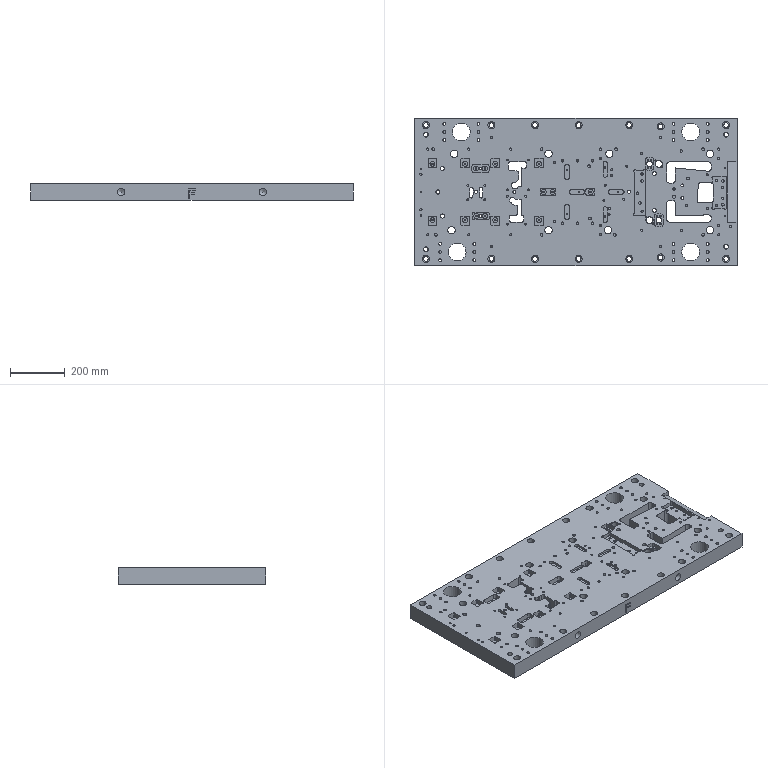Part | NX | features LIN_SOLID_COLOR 2 | 1 solid | 699 faces | box 1180 x 540 x 60 mm | volume 34145273 mm3 | cylinder 353 | plane 239 | cone 95 | spline 12 | commonest cylinder face diameters 8.5 x42 7 x32 10.002 x24 6.8 x21 5.2 x20 18 x20